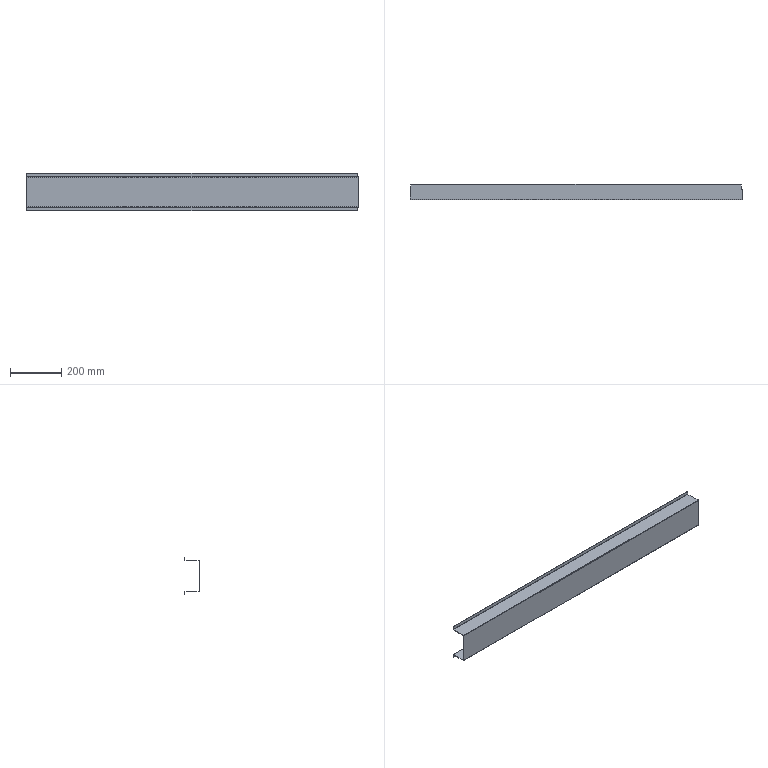Part | SolidWorks | features EdgeFlange 2, FlatPattern 1, ICE 1, SMBaseFlange 1, SheetMetal 1 | 1 solid | 38 faces | box 1298 x 58.8 x 147.6 mm | volume 406084 mm3 | plane 30 | cylinder 8 | commonest cylinder face diameters 0.9 x4 3.3 x4
STEP:
#1=CARTESIAN_POINT('',(646.8,57.15,60.));
#2=VERTEX_POINT('',#1);
#3=CARTESIAN_POINT('',(646.8,38.8,60.));
#4=VERTEX_POINT('',#3);
#5=CARTESIAN_POINT('',(646.8,58.8,60.));
#6=DIRECTION('',(0.,-1.,0.));
#7=VECTOR('',#6,1000.);
#8=LINE('',#5,#7);
#9=EDGE_CURVE('',#2,#4,#8,.T.);
#10=ORIENTED_EDGE('',*,*,#9,.F.);
#11=CARTESIAN_POINT('',(-646.8,57.15,60.));
#12=VERTEX_POINT('',#11);
#13=CARTESIAN_POINT('',(-648.8,57.15,60.));
#14=DIRECTION('',(1.,0.,0.));
#15=VECTOR('',#14,1000.);
#16=LINE('',#13,#15);
#17=EDGE_CURVE('',#12,#2,#16,.T.);
#18=ORIENTED_EDGE('',*,*,#17,.F.);
#19=CARTESIAN_POINT('',(-646.8,38.8,60.));
#20=VERTEX_POINT('',#19);
#21=CARTESIAN_POINT('',(-646.8,58.8,60.));
#22=DIRECTION('',(0.,1.,0.));
#23=VECTOR('',#22,1000.);
#24=LINE('',#21,#23);
#25=EDGE_CURVE('',#20,#12,#24,.T.);
#26=ORIENTED_EDGE('',*,*,#25,.F.);
#27=CARTESIAN_POINT('',(-648.8,38.8,60.));
#28=VERTEX_POINT('',#27);
#29=CARTESIAN_POINT('',(-648.8,38.8,60.));
#30=DIRECTION('',(1.,0.,0.));
#31=VECTOR('',#30,1000.);
#32=LINE('',#29,#31);
#33=EDGE_CURVE('',#28,#20,#32,.T.);
#34=ORIENTED_EDGE('',*,*,#33,.F.);
#35=CARTESIAN_POINT('',(-648.8,1.65,60.));
#36=VERTEX_POINT('',#35);
#37=CARTESIAN_POINT('',(-648.8,58.8,60.));
#38=DIRECTION('',(0.,-1.,0.));
#39=VECTOR('',#38,1000.);
#40=LINE('',#37,#39);
#41=EDGE_CURVE('',#28,#36,#40,.T.);
#42=ORIENTED_EDGE('',*,*,#41,.T.);
#43=CARTESIAN_POINT('',(648.8,1.65,60.));
#44=VERTEX_POINT('',#43);
#45=CARTESIAN_POINT('',(-648.8,1.65,60.));
#46=DIRECTION('',(-1.,0.,0.));
#47=VECTOR('',#46,1000.);
#48=LINE('',#45,#47);
#49=EDGE_CURVE('',#44,#36,#48,.T.);
#50=ORIENTED_EDGE('',*,*,#49,.F.);
#51=CARTESIAN_POINT('',(648.8,38.8,60.));
#52=VERTEX_POINT('',#51);
#53=CARTESIAN_POINT('',(648.8,58.8,60.));
#54=DIRECTION('',(0.,1.,0.));
#55=VECTOR('',#54,1000.);
#56=LINE('',#53,#55);
#57=EDGE_CURVE('',#44,#52,#56,.T.);
#58=ORIENTED_EDGE('',*,*,#57,.T.);
#59=CARTESIAN_POINT('',(-648.8,38.8,60.));
#60=DIRECTION('',(1.,0.,0.));
#61=VECTOR('',#60,1000.);
#62=LINE('',#59,#61);
#63=EDGE_CURVE('',#4,#52,#62,.T.);
#64=ORIENTED_EDGE('',*,*,#63,.F.);
#65=EDGE_LOOP('',(#10,#18,#26,#34,#42,#50,#58,#64));
#66=FACE_OUTER_BOUND('',#65,.T.);
#67=CARTESIAN_POINT('',(-648.8,58.8,60.));
#68=DIRECTION('',(0.,0.,-1.));
#69=DIRECTION('',(-1.,0.,0.));
#70=AXIS2_PLACEMENT_3D('',#67,#68,#69);
#71=PLANE('',#70);
#72=ADVANCED_FACE('',(#66),#71,.F.);
#73=CARTESIAN_POINT('',(-646.8,57.15,58.8));
#74=VERTEX_POINT('',#73);
#75=CARTESIAN_POINT('',(646.8,57.15,58.8));
#76=VERTEX_POINT('',#75);
#77=CARTESIAN_POINT('',(-648.8,57.15,58.8));
#78=DIRECTION('',(1.,0.,0.));
#79=VECTOR('',#78,1000.);
#80=LINE('',#77,#79);
#81=EDGE_CURVE('',#74,#76,#80,.T.);
#82=ORIENTED_EDGE('',*,*,#81,.T.);
#83=CARTESIAN_POINT('',(646.8,38.8,58.8));
#84=VERTEX_POINT('',#83);
#85=CARTESIAN_POINT('',(646.8,58.8,58.8));
#86=DIRECTION('',(0.,-1.,0.));
#87=VECTOR('',#86,1000.);
#88=LINE('',#85,#87);
#89=EDGE_CURVE('',#76,#84,#88,.T.);
#90=ORIENTED_EDGE('',*,*,#89,.T.);
#91=CARTESIAN_POINT('',(648.8,38.8,58.8));
#92=VERTEX_POINT('',#91);
#93=CARTESIAN_POINT('',(-648.8,38.8,58.8));
#94=DIRECTION('',(1.,0.,0.));
#95=VECTOR('',#94,1000.);
#96=LINE('',#93,#95);
#97=EDGE_CURVE('',#84,#92,#96,.T.);
#98=ORIENTED_EDGE('',*,*,#97,.T.);
#99=CARTESIAN_POINT('',(648.8,1.65,58.8));
#100=VERTEX_POINT('',#99);
#101=CARTESIAN_POINT('',(648.8,58.8,58.8));
#102=DIRECTION('',(0.,1.,0.));
#103=VECTOR('',#102,1000.);
#104=LINE('',#101,#103);
#105=EDGE_CURVE('',#100,#92,#104,.T.);
#106=ORIENTED_EDGE('',*,*,#105,.F.);
#107=CARTESIAN_POINT('',(-648.8,1.65,58.8));
#108=VERTEX_POINT('',#107);
#109=CARTESIAN_POINT('',(-648.8,1.65,58.8));
#110=DIRECTION('',(1.,0.,0.));
#111=VECTOR('',#110,1000.);
#112=LINE('',#109,#111);
#113=EDGE_CURVE('',#108,#100,#112,.T.);
#114=ORIENTED_EDGE('',*,*,#113,.F.);
#115=CARTESIAN_POINT('',(-648.8,38.8,58.8));
#116=VERTEX_POINT('',#115);
#117=CARTESIAN_POINT('',(-648.8,1.2,58.8));
#118=DIRECTION('',(0.,-1.,0.));
#119=VECTOR('',#118,1000.);
#120=LINE('',#117,#119);
#121=EDGE_CURVE('',#116,#108,#120,.T.);
#122=ORIENTED_EDGE('',*,*,#121,.F.);
#123=CARTESIAN_POINT('',(-646.8,38.8,58.8));
#124=VERTEX_POINT('',#123);
#125=CARTESIAN_POINT('',(-648.8,38.8,58.8));
#126=DIRECTION('',(1.,0.,0.));
#127=VECTOR('',#126,1000.);
#128=LINE('',#125,#127);
#129=EDGE_CURVE('',#116,#124,#128,.T.);
#130=ORIENTED_EDGE('',*,*,#129,.T.);
#131=CARTESIAN_POINT('',(-646.8,58.8,58.8));
#132=DIRECTION('',(0.,1.,0.));
#133=VECTOR('',#132,1000.);
#134=LINE('',#131,#133);
#135=EDGE_CURVE('',#124,#74,#134,.T.);
#136=ORIENTED_EDGE('',*,*,#135,.T.);
#137=EDGE_LOOP('',(#82,#90,#98,#106,#114,#122,#130,#136));
#138=FACE_OUTER_BOUND('',#137,.T.);
#139=CARTESIAN_POINT('',(-648.8,58.8,58.8));
#140=DIRECTION('',(0.,0.,-1.));
#141=DIRECTION('',(-1.,0.,0.));
#142=AXIS2_PLACEMENT_3D('',#139,#140,#141);
#143=PLANE('',#142);
#144=ADVANCED_FACE('',(#138),#143,.T.);
#145=CARTESIAN_POINT('',(646.8,38.8,-60.));
#146=VERTEX_POINT('',#145);
#147=CARTESIAN_POINT('',(646.8,57.15,-60.));
#148=VERTEX_POINT('',#147);
#149=CARTESIAN_POINT('',(646.8,58.8,-60.));
#150=DIRECTION('',(0.,1.,0.));
#151=VECTOR('',#150,1000.);
#152=LINE('',#149,#151);
#153=EDGE_CURVE('',#146,#148,#152,.T.);
#154=ORIENTED_EDGE('',*,*,#153,.F.);
#155=CARTESIAN_POINT('',(648.8,38.8,-60.));
#156=VERTEX_POINT('',#155);
#157=CARTESIAN_POINT('',(648.8,38.8,-60.));
#158=DIRECTION('',(-1.,0.,0.));
#159=VECTOR('',#158,1000.);
#160=LINE('',#157,#159);
#161=EDGE_CURVE('',#156,#146,#160,.T.);
#162=ORIENTED_EDGE('',*,*,#161,.F.);
#163=CARTESIAN_POINT('',(648.8,1.65,-60.));
#164=VERTEX_POINT('',#163);
#165=CARTESIAN_POINT('',(648.8,58.8,-60.));
#166=DIRECTION('',(0.,-1.,0.));
#167=VECTOR('',#166,1000.);
#168=LINE('',#165,#167);
#169=EDGE_CURVE('',#156,#164,#168,.T.);
#170=ORIENTED_EDGE('',*,*,#169,.T.);
#171=CARTESIAN_POINT('',(-648.8,1.65,-60.));
#172=VERTEX_POINT('',#171);
#173=CARTESIAN_POINT('',(648.8,1.65,-60.));
#174=DIRECTION('',(1.,0.,0.));
#175=VECTOR('',#174,1000.);
#176=LINE('',#173,#175);
#177=EDGE_CURVE('',#172,#164,#176,.T.);
#178=ORIENTED_EDGE('',*,*,#177,.F.);
#179=CARTESIAN_POINT('',(-648.8,38.8,-60.));
#180=VERTEX_POINT('',#179);
#181=CARTESIAN_POINT('',(-648.8,58.8,-60.));
#182=DIRECTION('',(0.,1.,0.));
#183=VECTOR('',#182,1000.);
#184=LINE('',#181,#183);
#185=EDGE_CURVE('',#172,#180,#184,.T.);
#186=ORIENTED_EDGE('',*,*,#185,.T.);
#187=CARTESIAN_POINT('',(-646.8,38.8,-60.));
#188=VERTEX_POINT('',#187);
#189=CARTESIAN_POINT('',(648.8,38.8,-60.));
#190=DIRECTION('',(-1.,0.,0.));
#191=VECTOR('',#190,1000.);
#192=LINE('',#189,#191);
#193=EDGE_CURVE('',#188,#180,#192,.T.);
#194=ORIENTED_EDGE('',*,*,#193,.F.);
#195=CARTESIAN_POINT('',(-646.8,57.15,-60.));
#196=VERTEX_POINT('',#195);
#197=CARTESIAN_POINT('',(-646.8,58.8,-60.));
#198=DIRECTION('',(0.,-1.,0.));
#199=VECTOR('',#198,1000.);
#200=LINE('',#197,#199);
#201=EDGE_CURVE('',#196,#188,#200,.T.);
#202=ORIENTED_EDGE('',*,*,#201,.F.);
#203=CARTESIAN_POINT('',(648.8,57.15,-60.));
#204=DIRECTION('',(-1.,0.,0.));
#205=VECTOR('',#204,1000.);
#206=LINE('',#203,#205);
#207=EDGE_CURVE('',#148,#196,#206,.T.);
#208=ORIENTED_EDGE('',*,*,#207,.F.);
#209=EDGE_LOOP('',(#154,#162,#170,#178,#186,#194,#202,#208));
#210=FACE_OUTER_BOUND('',#209,.T.);
#211=CARTESIAN_POINT('',(648.8,58.8,-60.));
#212=DIRECTION('',(0.,0.,1.));
#213=DIRECTION('',(0.,-1.,0.));
#214=AXIS2_PLACEMENT_3D('',#211,#212,#213);
#215=PLANE('',#214);
#216=ADVANCED_FACE('',(#210),#215,.F.);
#217=CARTESIAN_POINT('',(648.8,38.8,-58.8));
#218=VERTEX_POINT('',#217);
#219=CARTESIAN_POINT('',(646.8,38.8,-58.8));
#220=VERTEX_POINT('',#219);
#221=CARTESIAN_POINT('',(648.8,38.8,-58.8));
#222=DIRECTION('',(-1.,0.,0.));
#223=VECTOR('',#222,1000.);
#224=LINE('',#221,#223);
#225=EDGE_CURVE('',#218,#220,#224,.T.);
#226=ORIENTED_EDGE('',*,*,#225,.T.);
#227=CARTESIAN_POINT('',(646.8,57.15,-58.8));
#228=VERTEX_POINT('',#227);
#229=CARTESIAN_POINT('',(646.8,58.8,-58.8));
#230=DIRECTION('',(0.,1.,0.));
#231=VECTOR('',#230,1000.);
#232=LINE('',#229,#231);
#233=EDGE_CURVE('',#220,#228,#232,.T.);
#234=ORIENTED_EDGE('',*,*,#233,.T.);
#235=CARTESIAN_POINT('',(-646.8,57.15,-58.8));
#236=VERTEX_POINT('',#235);
#237=CARTESIAN_POINT('',(648.8,57.15,-58.8));
#238=DIRECTION('',(-1.,0.,0.));
#239=VECTOR('',#238,1000.);
#240=LINE('',#237,#239);
#241=EDGE_CURVE('',#228,#236,#240,.T.);
#242=ORIENTED_EDGE('',*,*,#241,.T.);
#243=CARTESIAN_POINT('',(-646.8,38.8,-58.8));
#244=VERTEX_POINT('',#243);
#245=CARTESIAN_POINT('',(-646.8,58.8,-58.8));
#246=DIRECTION('',(0.,-1.,0.));
#247=VECTOR('',#246,1000.);
#248=LINE('',#245,#247);
#249=EDGE_CURVE('',#236,#244,#248,.T.);
#250=ORIENTED_EDGE('',*,*,#249,.T.);
#251=CARTESIAN_POINT('',(-648.8,38.8,-58.8));
#252=VERTEX_POINT('',#251);
#253=CARTESIAN_POINT('',(648.8,38.8,-58.8));
#254=DIRECTION('',(-1.,0.,0.));
#255=VECTOR('',#254,1000.);
#256=LINE('',#253,#255);
#257=EDGE_CURVE('',#244,#252,#256,.T.);
#258=ORIENTED_EDGE('',*,*,#257,.T.);
#259=CARTESIAN_POINT('',(-648.8,1.65,-58.8));
#260=VERTEX_POINT('',#259);
#261=CARTESIAN_POINT('',(-648.8,58.8,-58.8));
#262=DIRECTION('',(0.,1.,0.));
#263=VECTOR('',#262,1000.);
#264=LINE('',#261,#263);
#265=EDGE_CURVE('',#260,#252,#264,.T.);
#266=ORIENTED_EDGE('',*,*,#265,.F.);
#267=CARTESIAN_POINT('',(648.8,1.65,-58.8));
#268=VERTEX_POINT('',#267);
#269=CARTESIAN_POINT('',(648.8,1.65,-58.8));
#270=DIRECTION('',(-1.,0.,0.));
#271=VECTOR('',#270,1000.);
#272=LINE('',#269,#271);
#273=EDGE_CURVE('',#268,#260,#272,.T.);
#274=ORIENTED_EDGE('',*,*,#273,.F.);
#275=CARTESIAN_POINT('',(648.8,1.2,-58.8));
#276=DIRECTION('',(0.,-1.,0.));
#277=VECTOR('',#276,1000.);
#278=LINE('',#275,#277);
#279=EDGE_CURVE('',#218,#268,#278,.T.);
#280=ORIENTED_EDGE('',*,*,#279,.F.);
#281=EDGE_LOOP('',(#226,#234,#242,#250,#258,#266,#274,#280));
#282=FACE_OUTER_BOUND('',#281,.T.);
#283=CARTESIAN_POINT('',(648.8,58.8,-58.8));
#284=DIRECTION('',(0.,0.,1.));
#285=DIRECTION('',(0.,-1.,0.));
#286=AXIS2_PLACEMENT_3D('',#283,#284,#285);
#287=PLANE('',#286);
#288=ADVANCED_FACE('',(#282),#287,.T.);
#289=ORIENTED_EDGE('',*,*,#241,.F.);
#290=CARTESIAN_POINT('',(646.8,58.8,-60.45));
#291=VERTEX_POINT('',#290);
#292=CARTESIAN_POINT('',(646.8,57.15,-60.45));
#293=DIRECTION('',(-1.,0.,0.));
#294=DIRECTION('',(0.,0.,-1.));
#295=AXIS2_PLACEMENT_3D('',#292,#293,#294);
#296=CIRCLE('',#295,1.65);
#297=EDGE_CURVE('',#228,#291,#296,.T.);
#298=ORIENTED_EDGE('',*,*,#297,.T.);
#299=CARTESIAN_POINT('',(-646.8,58.8,-60.45));
#300=VERTEX_POINT('',#299);
#301=CARTESIAN_POINT('',(648.8,58.8,-60.45));
#302=DIRECTION('',(1.,0.,0.));
#303=VECTOR('',#302,1000.);
#304=LINE('',#301,#303);
#305=EDGE_CURVE('',#300,#291,#304,.T.);
#306=ORIENTED_EDGE('',*,*,#305,.F.);
#307=CARTESIAN_POINT('',(-646.8,57.15,-60.45));
#308=DIRECTION('',(1.,0.,0.));
#309=DIRECTION('',(0.,0.,1.));
#310=AXIS2_PLACEMENT_3D('',#307,#308,#309);
#311=CIRCLE('',#310,1.65);
#312=EDGE_CURVE('',#300,#236,#311,.T.);
#313=ORIENTED_EDGE('',*,*,#312,.T.);
#314=EDGE_LOOP('',(#289,#298,#306,#313));
#315=FACE_OUTER_BOUND('',#314,.T.);
#316=CARTESIAN_POINT('',(648.8,57.15,-60.45));
#317=DIRECTION('',(1.,0.,0.));
#318=DIRECTION('',(0.,1.,0.));
#319=AXIS2_PLACEMENT_3D('',#316,#317,#318);
#320=CYLINDRICAL_SURFACE('',#319,1.65);
#321=ADVANCED_FACE('',(#315),#320,.T.);
#322=CARTESIAN_POINT('',(646.8,57.6,-60.45));
#323=VERTEX_POINT('',#322);
#324=CARTESIAN_POINT('',(646.8,57.15,-60.45));
#325=DIRECTION('',(-1.,0.,0.));
#326=DIRECTION('',(0.,0.,-1.));
#327=AXIS2_PLACEMENT_3D('',#324,#325,#326);
#328=CIRCLE('',#327,0.45);
#329=EDGE_CURVE('',#148,#323,#328,.T.);
#330=ORIENTED_EDGE('',*,*,#329,.F.);
#331=ORIENTED_EDGE('',*,*,#207,.T.);
#332=CARTESIAN_POINT('',(-646.8,57.6,-60.45));
#333=VERTEX_POINT('',#332);
#334=CARTESIAN_POINT('',(-646.8,57.15,-60.45));
#335=DIRECTION('',(1.,0.,0.));
#336=DIRECTION('',(0.,0.,1.));
#337=AXIS2_PLACEMENT_3D('',#334,#335,#336);
#338=CIRCLE('',#337,0.45);
#339=EDGE_CURVE('',#333,#196,#338,.T.);
#340=ORIENTED_EDGE('',*,*,#339,.F.);
#341=CARTESIAN_POINT('',(-648.8,57.6,-60.45));
#342=DIRECTION('',(1.,0.,0.));
#343=VECTOR('',#342,1000.);
#344=LINE('',#341,#343);
#345=EDGE_CURVE('',#333,#323,#344,.T.);
#346=ORIENTED_EDGE('',*,*,#345,.T.);
#347=EDGE_LOOP('',(#330,#331,#340,#346));
#348=FACE_OUTER_BOUND('',#347,.T.);
#349=CARTESIAN_POINT('',(648.8,57.15,-60.45));
#350=DIRECTION('',(1.,0.,0.));
#351=DIRECTION('',(0.,1.,0.));
#352=AXIS2_PLACEMENT_3D('',#349,#350,#351);
#353=CYLINDRICAL_SURFACE('',#352,0.45);
#354=ADVANCED_FACE('',(#348),#353,.F.);
#355=ORIENTED_EDGE('',*,*,#305,.T.);
#356=CARTESIAN_POINT('',(646.8,58.8,-73.8));
#357=VERTEX_POINT('',#356);
#358=CARTESIAN_POINT('',(646.8,58.8,140.));
#359=DIRECTION('',(0.,0.,-1.));
#360=VECTOR('',#359,1000.);
#361=LINE('',#358,#360);
#362=EDGE_CURVE('',#291,#357,#361,.T.);
#363=ORIENTED_EDGE('',*,*,#362,.T.);
#364=CARTESIAN_POINT('',(-646.8,58.8,-73.8));
#365=VERTEX_POINT('',#364);
#366=CARTESIAN_POINT('',(648.8,58.8,-73.8));
#367=DIRECTION('',(1.,0.,0.));
#368=VECTOR('',#367,1000.);
#369=LINE('',#366,#368);
#370=EDGE_CURVE('',#365,#357,#369,.T.);
#371=ORIENTED_EDGE('',*,*,#370,.F.);
#372=CARTESIAN_POINT('',(-646.8,58.8,140.));
#373=DIRECTION('',(0.,0.,-1.));
#374=VECTOR('',#373,1000.);
#375=LINE('',#372,#374);
#376=EDGE_CURVE('',#300,#365,#375,.T.);
#377=ORIENTED_EDGE('',*,*,#376,.F.);
#378=EDGE_LOOP('',(#355,#363,#371,#377));
#379=FACE_OUTER_BOUND('',#378,.T.);
#380=CARTESIAN_POINT('',(648.8,58.8,-60.));
#381=DIRECTION('',(0.,1.,0.));
#382=DIRECTION('',(0.,0.,1.));
#383=AXIS2_PLACEMENT_3D('',#380,#381,#382);
#384=PLANE('',#383);
#385=ADVANCED_FACE('',(#379),#384,.T.);
#386=CARTESIAN_POINT('',(646.8,57.6,-73.8));
#387=VERTEX_POINT('',#386);
#388=CARTESIAN_POINT('',(646.8,57.6,-60.));
#389=DIRECTION('',(0.,0.,-1.));
#390=VECTOR('',#389,1000.);
#391=LINE('',#388,#390);
#392=EDGE_CURVE('',#323,#387,#391,.T.);
#393=ORIENTED_EDGE('',*,*,#392,.F.);
#394=ORIENTED_EDGE('',*,*,#345,.F.);
#395=CARTESIAN_POINT('',(-646.8,57.6,-73.8));
#396=VERTEX_POINT('',#395);
#397=CARTESIAN_POINT('',(-646.8,57.6,-60.));
#398=DIRECTION('',(0.,0.,1.));
#399=VECTOR('',#398,1000.);
#400=LINE('',#397,#399);
#401=EDGE_CURVE('',#396,#333,#400,.T.);
#402=ORIENTED_EDGE('',*,*,#401,.F.);
#403=CARTESIAN_POINT('',(648.8,57.6,-73.8));
#404=DIRECTION('',(1.,0.,0.));
#405=VECTOR('',#404,1000.);
#406=LINE('',#403,#405);
#407=EDGE_CURVE('',#396,#387,#406,.T.);
#408=ORIENTED_EDGE('',*,*,#407,.T.);
#409=EDGE_LOOP('',(#393,#394,#402,#408));
#410=FACE_OUTER_BOUND('',#409,.T.);
#411=CARTESIAN_POINT('',(648.8,57.6,-60.));
#412=DIRECTION('',(0.,1.,0.));
#413=DIRECTION('',(0.,0.,1.));
#414=AXIS2_PLACEMENT_3D('',#411,#412,#413);
#415=PLANE('',#414);
#416=ADVANCED_FACE('',(#410),#415,.F.);
#417=ORIENTED_EDGE('',*,*,#370,.T.);
#418=CARTESIAN_POINT('',(646.8,58.8,-73.8));
#419=DIRECTION('',(0.,-1.,0.));
#420=VECTOR('',#419,1000.);
#421=LINE('',#418,#420);
#422=EDGE_CURVE('',#357,#387,#421,.T.);
#423=ORIENTED_EDGE('',*,*,#422,.T.);
#424=ORIENTED_EDGE('',*,*,#407,.F.);
#425=CARTESIAN_POINT('',(-646.8,58.8,-73.8));
#426=DIRECTION('',(0.,1.,0.));
#427=VECTOR('',#426,1000.);
#428=LINE('',#425,#427);
#429=EDGE_CURVE('',#396,#365,#428,.T.);
#430=ORIENTED_EDGE('',*,*,#429,.T.);
#431=EDGE_LOOP('',(#417,#423,#424,#430));
#432=FACE_OUTER_BOUND('',#431,.T.);
#433=CARTESIAN_POINT('',(648.8,58.8,-73.8));
#434=DIRECTION('',(0.,0.,-1.));
#435=DIRECTION('',(0.,1.,0.));
#436=AXIS2_PLACEMENT_3D('',#433,#434,#435);
#437=PLANE('',#436);
#438=ADVANCED_FACE('',(#432),#437,.T.);
#439=CARTESIAN_POINT('',(-646.8,58.8,60.45));
#440=VERTEX_POINT('',#439);
#441=CARTESIAN_POINT('',(646.8,58.8,60.45));
#442=VERTEX_POINT('',#441);
#443=CARTESIAN_POINT('',(648.8,58.8,60.45));
#444=DIRECTION('',(1.,0.,0.));
#445=VECTOR('',#444,1000.);
#446=LINE('',#443,#445);
#447=EDGE_CURVE('',#440,#442,#446,.T.);
#448=ORIENTED_EDGE('',*,*,#447,.T.);
#449=CARTESIAN_POINT('',(646.8,57.15,60.45));
#450=DIRECTION('',(-1.,0.,0.));
#451=DIRECTION('',(0.,0.,-1.));
#452=AXIS2_PLACEMENT_3D('',#449,#450,#451);
#453=CIRCLE('',#452,1.65);
#454=EDGE_CURVE('',#442,#76,#453,.T.);
#455=ORIENTED_EDGE('',*,*,#454,.T.);
#456=ORIENTED_EDGE('',*,*,#81,.F.);
#457=CARTESIAN_POINT('',(-646.8,57.15,60.45));
#458=DIRECTION('',(1.,0.,0.));
#459=DIRECTION('',(0.,0.,1.));
#460=AXIS2_PLACEMENT_3D('',#457,#458,#459);
#461=CIRCLE('',#460,1.65);
#462=EDGE_CURVE('',#74,#440,#461,.T.);
#463=ORIENTED_EDGE('',*,*,#462,.T.);
#464=EDGE_LOOP('',(#448,#455,#456,#463));
#465=FACE_OUTER_BOUND('',#464,.T.);
#466=CARTESIAN_POINT('',(-648.8,57.15,60.45));
#467=DIRECTION('',(-1.,0.,0.));
#468=DIRECTION('',(0.,1.,0.));
#469=AXIS2_PLACEMENT_3D('',#466,#467,#468);
#470=CYLINDRICAL_SURFACE('',#469,1.65);
#471=ADVANCED_FACE('',(#465),#470,.T.);
#472=CARTESIAN_POINT('',(646.8,57.6,60.45));
#473=VERTEX_POINT('',#472);
#474=CARTESIAN_POINT('',(646.8,57.15,60.45));
#475=DIRECTION('',(-1.,0.,0.));
#476=DIRECTION('',(0.,0.,-1.));
#477=AXIS2_PLACEMENT_3D('',#474,#475,#476);
#478=CIRCLE('',#477,0.45);
#479=EDGE_CURVE('',#473,#2,#478,.T.);
#480=ORIENTED_EDGE('',*,*,#479,.F.);
#481=CARTESIAN_POINT('',(-646.8,57.6,60.45));
#482=VERTEX_POINT('',#481);
#483=CARTESIAN_POINT('',(648.8,57.6,60.45));
#484=DIRECTION('',(-1.,0.,0.));
#485=VECTOR('',#484,1000.);
#486=LINE('',#483,#485);
#487=EDGE_CURVE('',#473,#482,#486,.T.);
#488=ORIENTED_EDGE('',*,*,#487,.T.);
#489=CARTESIAN_POINT('',(-646.8,57.15,60.45));
#490=DIRECTION('',(1.,0.,0.));
#491=DIRECTION('',(0.,0.,1.));
#492=AXIS2_PLACEMENT_3D('',#489,#490,#491);
#493=CIRCLE('',#492,0.45);
#494=EDGE_CURVE('',#12,#482,#493,.T.);
#495=ORIENTED_EDGE('',*,*,#494,.F.);
#496=ORIENTED_EDGE('',*,*,#17,.T.);
#497=EDGE_LOOP('',(#480,#488,#495,#496));
#498=FACE_OUTER_BOUND('',#497,.T.);
#499=CARTESIAN_POINT('',(-648.8,57.15,60.45));
#500=DIRECTION('',(-1.,0.,0.));
#501=DIRECTION('',(0.,1.,0.));
#502=AXIS2_PLACEMENT_3D('',#499,#500,#501);
#503=CYLINDRICAL_SURFACE('',#502,0.45);
#504=ADVANCED_FACE('',(#498),#503,.F.);
#505=CARTESIAN_POINT('',(646.8,58.8,73.8));
#506=VERTEX_POINT('',#505);
#507=CARTESIAN_POINT('',(646.8,58.8,140.));
#508=DIRECTION('',(0.,0.,-1.));
#509=VECTOR('',#508,1000.);
#510=LINE('',#507,#509);
#511=EDGE_CURVE('',#506,#442,#510,.T.);
#512=ORIENTED_EDGE('',*,*,#511,.T.);
#513=ORIENTED_EDGE('',*,*,#447,.F.);
#514=CARTESIAN_POINT('',(-646.8,58.8,73.8));
#515=VERTEX_POINT('',#514);
#516=CARTESIAN_POINT('',(-646.8,58.8,140.));
#517=DIRECTION('',(0.,0.,-1.));
#518=VECTOR('',#517,1000.);
#519=LINE('',#516,#518);
#520=EDGE_CURVE('',#515,#440,#519,.T.);
#521=ORIENTED_EDGE('',*,*,#520,.F.);
#522=CARTESIAN_POINT('',(648.8,58.8,73.8));
#523=DIRECTION('',(-1.,0.,0.));
#524=VECTOR('',#523,1000.);
#525=LINE('',#522,#524);
#526=EDGE_CURVE('',#506,#515,#525,.T.);
#527=ORIENTED_EDGE('',*,*,#526,.F.);
#528=EDGE_LOOP('',(#512,#513,#521,#527));
#529=FACE_OUTER_BOUND('',#528,.T.);
#530=CARTESIAN_POINT('',(648.8,58.8,73.8));
#531=DIRECTION('',(0.,-1.,0.));
#532=DIRECTION('',(0.,0.,-1.));
#533=AXIS2_PLACEMENT_3D('',#530,#531,#532);
#534=PLANE('',#533);
#535=ADVANCED_FACE('',(#529),#534,.F.);
#536=ORIENTED_EDGE('',*,*,#487,.F.);
#537=CARTESIAN_POINT('',(646.8,57.6,73.8));
#538=VERTEX_POINT('',#537);
#539=CARTESIAN_POINT('',(646.8,57.6,73.8));
#540=DIRECTION('',(0.,0.,1.));
#541=VECTOR('',#540,1000.);
#542=LINE('',#539,#541);
#543=EDGE_CURVE('',#473,#538,#542,.T.);
#544=ORIENTED_EDGE('',*,*,#543,.T.);
#545=CARTESIAN_POINT('',(-646.8,57.6,73.8));
#546=VERTEX_POINT('',#545);
#547=CARTESIAN_POINT('',(648.8,57.6,73.8));
#548=DIRECTION('',(-1.,0.,0.));
#549=VECTOR('',#548,1000.);
#550=LINE('',#547,#549);
#551=EDGE_CURVE('',#538,#546,#550,.T.);
#552=ORIENTED_EDGE('',*,*,#551,.T.);
#553=CARTESIAN_POINT('',(-646.8,57.6,73.8));
#554=DIRECTION('',(0.,0.,-1.));
#555=VECTOR('',#554,1000.);
#556=LINE('',#553,#555);
#557=EDGE_CURVE('',#546,#482,#556,.T.);
#558=ORIENTED_EDGE('',*,*,#557,.T.);
#559=EDGE_LOOP('',(#536,#544,#552,#558));
#560=FACE_OUTER_BOUND('',#559,.T.);
#561=CARTESIAN_POINT('',(648.8,57.6,73.8));
#562=DIRECTION('',(0.,-1.,0.));
#563=DIRECTION('',(0.,0.,-1.));
#564=AXIS2_PLACEMENT_3D('',#561,#562,#563);
#565=PLANE('',#564);
#566=ADVANCED_FACE('',(#560),#565,.T.);
#567=ORIENTED_EDGE('',*,*,#551,.F.);
#568=CARTESIAN_POINT('',(646.8,58.8,73.8));
#569=DIRECTION('',(0.,1.,0.));
#570=VECTOR('',#569,1000.);
#571=LINE('',#568,#570);
#572=EDGE_CURVE('',#538,#506,#571,.T.);
#573=ORIENTED_EDGE('',*,*,#572,.T.);
#574=ORIENTED_EDGE('',*,*,#526,.T.);
#575=CARTESIAN_POINT('',(-646.8,58.8,73.8));
#576=DIRECTION('',(0.,-1.,0.));
#577=VECTOR('',#576,1000.);
#578=LINE('',#575,#577);
#579=EDGE_CURVE('',#515,#546,#578,.T.);
#580=ORIENTED_EDGE('',*,*,#579,.T.);
#581=EDGE_LOOP('',(#567,#573,#574,#580));
#582=FACE_OUTER_BOUND('',#581,.T.);
#583=CARTESIAN_POINT('',(648.8,58.8,73.8));
#584=DIRECTION('',(0.,0.,1.));
#585=DIRECTION('',(0.,-1.,0.));
#586=AXIS2_PLACEMENT_3D('',#583,#584,#585);
#587=PLANE('',#586);
#588=ADVANCED_FACE('',(#582),#587,.T.);
#589=CARTESIAN_POINT('',(648.8,38.8,140.));
#590=DIRECTION('',(0.,0.,-1.));
#591=VECTOR('',#590,1000.);
#592=LINE('',#589,#591);
#593=EDGE_CURVE('',#52,#92,#592,.T.);
#594=ORIENTED_EDGE('',*,*,#593,.F.);
#595=ORIENTED_EDGE('',*,*,#57,.F.);
#596=CARTESIAN_POINT('',(648.8,1.65,58.8));
#597=DIRECTION('',(0.,0.,1.));
#598=VECTOR('',#597,1000.);
#599=LINE('',#596,#598);
#600=EDGE_CURVE('',#100,#44,#599,.T.);
#601=ORIENTED_EDGE('',*,*,#600,.F.);
#602=ORIENTED_EDGE('',*,*,#105,.T.);
#603=EDGE_LOOP('',(#594,#595,#601,#602));
#604=FACE_OUTER_BOUND('',#603,.T.);
#605=CARTESIAN_POINT('',(648.8,58.8,60.));
#606=DIRECTION('',(-1.,0.,0.));
#607=DIRECTION('',(0.,0.,1.));
#608=AXIS2_PLACEMENT_3D('',#605,#606,#607);
#609=PLANE('',#608);
#610=ADVANCED_FACE('',(#604),#609,.F.);
#611=CARTESIAN_POINT('',(648.8,38.8,-60.));
#612=DIRECTION('',(0.,0.,-1.));
#613=VECTOR('',#612,1000.);
#614=LINE('',#611,#613);
#615=EDGE_CURVE('',#218,#156,#614,.T.);
#616=ORIENTED_EDGE('',*,*,#615,.F.);
#617=ORIENTED_EDGE('',*,*,#279,.T.);
#618=CARTESIAN_POINT('',(648.8,1.65,-60.));
#619=DIRECTION('',(0.,0.,-1.));
#620=VECTOR('',#619,1000.);
#621=LINE('',#618,#620);
#622=EDGE_CURVE('',#268,#164,#621,.T.);
#623=ORIENTED_EDGE('',*,*,#622,.T.);
#624=ORIENTED_EDGE('',*,*,#169,.F.);
#625=EDGE_LOOP('',(#616,#617,#623,#624));
#626=FACE_OUTER_BOUND('',#625,.T.);
#627=CARTESIAN_POINT('',(648.8,1.2,-60.));
#628=DIRECTION('',(-1.,0.,0.));
#629=DIRECTION('',(0.,0.,1.));
#630=AXIS2_PLACEMENT_3D('',#627,#628,#629);
#631=PLANE('',#630);
#632=ADVANCED_FACE('',(#626),#631,.F.);
#633=CARTESIAN_POINT('',(-648.8,38.8,140.));
#634=DIRECTION('',(0.,0.,-1.));
#635=VECTOR('',#634,1000.);
#636=LINE('',#633,#635);
#637=EDGE_CURVE('',#28,#116,#636,.T.);
#638=ORIENTED_EDGE('',*,*,#637,.T.);
#639=ORIENTED_EDGE('',*,*,#121,.T.);
#640=CARTESIAN_POINT('',(-648.8,1.65,60.));
#641=DIRECTION('',(0.,0.,1.));
#642=VECTOR('',#641,1000.);
#643=LINE('',#640,#642);
#644=EDGE_CURVE('',#108,#36,#643,.T.);
#645=ORIENTED_EDGE('',*,*,#644,.T.);
#646=ORIENTED_EDGE('',*,*,#41,.F.);
#647=EDGE_LOOP('',(#638,#639,#645,#646));
#648=FACE_OUTER_BOUND('',#647,.T.);
#649=CARTESIAN_POINT('',(-648.8,1.2,60.));
#650=DIRECTION('',(1.,0.,0.));
#651=DIRECTION('',(0.,0.,-1.));
#652=AXIS2_PLACEMENT_3D('',#649,#650,#651);
#653=PLANE('',#652);
#654=ADVANCED_FACE('',(#648),#653,.F.);
#655=CARTESIAN_POINT('',(-648.8,38.8,140.));
#656=DIRECTION('',(0.,0.,-1.));
#657=VECTOR('',#656,1000.);
#658=LINE('',#655,#657);
#659=EDGE_CURVE('',#252,#180,#658,.T.);
#660=ORIENTED_EDGE('',*,*,#659,.T.);
#661=ORIENTED_EDGE('',*,*,#185,.F.);
#662=CARTESIAN_POINT('',(-648.8,1.65,-58.8));
#663=DIRECTION('',(0.,0.,-1.));
#664=VECTOR('',#663,1000.);
#665=LINE('',#662,#664);
#666=EDGE_CURVE('',#260,#172,#665,.T.);
#667=ORIENTED_EDGE('',*,*,#666,.F.);
#668=ORIENTED_EDGE('',*,*,#265,.T.);
#669=EDGE_LOOP('',(#660,#661,#667,#668));
#670=FACE_OUTER_BOUND('',#669,.T.);
#671=CARTESIAN_POINT('',(-648.8,58.8,-60.));
#672=DIRECTION('',(1.,0.,0.));
#673=DIRECTION('',(0.,0.,-1.));
#674=AXIS2_PLACEMENT_3D('',#671,#672,#673);
#675=PLANE('',#674);
#676=ADVANCED_FACE('',(#670),#675,.F.);
#677=CARTESIAN_POINT('',(-648.8,1.2,58.35));
#678=VERTEX_POINT('',#677);
#679=CARTESIAN_POINT('',(-648.8,0.,58.35));
#680=VERTEX_POINT('',#679);
#681=CARTESIAN_POINT('',(-648.8,1.2,58.35));
#682=DIRECTION('',(0.,-1.,0.));
#683=VECTOR('',#682,1000.);
#684=LINE('',#681,#683);
#685=EDGE_CURVE('',#678,#680,#684,.T.);
#686=ORIENTED_EDGE('',*,*,#685,.F.);
#687=CARTESIAN_POINT('',(-648.8,1.2,-58.35));
#688=VERTEX_POINT('',#687);
#689=CARTESIAN_POINT('',(-648.8,1.2,-60.));
#690=DIRECTION('',(0.,0.,1.));
#691=VECTOR('',#690,1000.);
#692=LINE('',#689,#691);
#693=EDGE_CURVE('',#688,#678,#692,.T.);
#694=ORIENTED_EDGE('',*,*,#693,.F.);
#695=CARTESIAN_POINT('',(-648.8,0.,-58.35));
#696=VERTEX_POINT('',#695);
#697=CARTESIAN_POINT('',(-648.8,1.2,-58.35));
#698=DIRECTION('',(0.,-1.,0.));
#699=VECTOR('',#698,1000.);
#700=LINE('',#697,#699);
#701=EDGE_CURVE('',#688,#696,#700,.T.);
#702=ORIENTED_EDGE('',*,*,#701,.T.);
#703=CARTESIAN_POINT('',(-648.8,0.,-60.));
#704=DIRECTION('',(0.,0.,1.));
#705=VECTOR('',#704,1000.);
#706=LINE('',#703,#705);
#707=EDGE_CURVE('',#696,#680,#706,.T.);
#708=ORIENTED_EDGE('',*,*,#707,.T.);
#709=EDGE_LOOP('',(#686,#694,#702,#708));
#710=FACE_OUTER_BOUND('',#709,.T.);
#711=CARTESIAN_POINT('',(-648.8,1.2,-60.));
#712=DIRECTION('',(1.,0.,0.));
#713=DIRECTION('',(0.,0.,-1.));
#714=AXIS2_PLACEMENT_3D('',#711,#712,#713);
#715=PLANE('',#714);
#716=ADVANCED_FACE('',(#710),#715,.F.);
#717=CARTESIAN_POINT('',(648.8,1.2,58.35));
#718=VERTEX_POINT('',#717);
#719=CARTESIAN_POINT('',(648.8,0.,58.35));
#720=VERTEX_POINT('',#719);
#721=CARTESIAN_POINT('',(648.8,1.2,58.35));
#722=DIRECTION('',(0.,-1.,0.));
#723=VECTOR('',#722,1000.);
#724=LINE('',#721,#723);
#725=EDGE_CURVE('',#718,#720,#724,.T.);
#726=ORIENTED_EDGE('',*,*,#725,.T.);
#727=CARTESIAN_POINT('',(648.8,0.,-58.35));
#728=VERTEX_POINT('',#727);
#729=CARTESIAN_POINT('',(648.8,0.,-60.));
#730=DIRECTION('',(0.,0.,-1.));
#731=VECTOR('',#730,1000.);
#732=LINE('',#729,#731);
#733=EDGE_CURVE('',#720,#728,#732,.T.);
#734=ORIENTED_EDGE('',*,*,#733,.T.);
#735=CARTESIAN_POINT('',(648.8,1.2,-58.35));
#736=VERTEX_POINT('',#735);
#737=CARTESIAN_POINT('',(648.8,1.2,-58.35));
#738=DIRECTION('',(0.,-1.,0.));
#739=VECTOR('',#738,1000.);
#740=LINE('',#737,#739);
#741=EDGE_CURVE('',#736,#728,#740,.T.);
#742=ORIENTED_EDGE('',*,*,#741,.F.);
#743=CARTESIAN_POINT('',(648.8,1.2,-60.));
#744=DIRECTION('',(0.,0.,-1.));
#745=VECTOR('',#744,1000.);
#746=LINE('',#743,#745);
#747=EDGE_CURVE('',#718,#736,#746,.T.);
#748=ORIENTED_EDGE('',*,*,#747,.F.);
#749=EDGE_LOOP('',(#726,#734,#742,#748));
#750=FACE_OUTER_BOUND('',#749,.T.);
#751=CARTESIAN_POINT('',(648.8,1.2,-60.));
#752=DIRECTION('',(-1.,0.,0.));
#753=DIRECTION('',(0.,0.,1.));
#754=AXIS2_PLACEMENT_3D('',#751,#752,#753);
#755=PLANE('',#754);
#756=ADVANCED_FACE('',(#750),#755,.F.);
#757=ORIENTED_EDGE('',*,*,#693,.T.);
#758=CARTESIAN_POINT('',(648.8,1.2,58.35));
#759=DIRECTION('',(-1.,0.,0.));
#760=VECTOR('',#759,1000.);
#761=LINE('',#758,#760);
#762=EDGE_CURVE('',#718,#678,#761,.T.);
#763=ORIENTED_EDGE('',*,*,#762,.F.);
#764=ORIENTED_EDGE('',*,*,#747,.T.);
#765=CARTESIAN_POINT('',(-648.8,1.2,-58.35));
#766=DIRECTION('',(1.,0.,0.));
#767=VECTOR('',#766,1000.);
#768=LINE('',#765,#767);
#769=EDGE_CURVE('',#688,#736,#768,.T.);
#770=ORIENTED_EDGE('',*,*,#769,.F.);
#771=EDGE_LOOP('',(#757,#763,#764,#770));
#772=FACE_OUTER_BOUND('',#771,.T.);
#773=CARTESIAN_POINT('',(-648.8,1.2,60.));
#774=DIRECTION('',(0.,1.,0.));
#775=DIRECTION('',(0.,0.,1.));
#776=AXIS2_PLACEMENT_3D('',#773,#774,#775);
#777=PLANE('',#776);
#778=ADVANCED_FACE('',(#772),#777,.T.);
#779=CARTESIAN_POINT('',(648.8,0.,58.35));
#780=DIRECTION('',(-1.,0.,0.));
#781=VECTOR('',#780,1000.);
#782=LINE('',#779,#781);
#783=EDGE_CURVE('',#720,#680,#782,.T.);
#784=ORIENTED_EDGE('',*,*,#783,.T.);
#785=ORIENTED_EDGE('',*,*,#707,.F.);
#786=CARTESIAN_POINT('',(-648.8,0.,-58.35));
#787=DIRECTION('',(1.,0.,0.));
#788=VECTOR('',#787,1000.);
#789=LINE('',#786,#788);
#790=EDGE_CURVE('',#696,#728,#789,.T.);
#791=ORIENTED_EDGE('',*,*,#790,.T.);
#792=ORIENTED_EDGE('',*,*,#733,.F.);
#793=EDGE_LOOP('',(#784,#785,#791,#792));
#794=FACE_OUTER_BOUND('',#793,.T.);
#795=CARTESIAN_POINT('',(-648.8,0.,60.));
#796=DIRECTION('',(0.,1.,0.));
#797=DIRECTION('',(0.,0.,1.));
#798=AXIS2_PLACEMENT_3D('',#795,#796,#797);
#799=PLANE('',#798);
#800=ADVANCED_FACE('',(#794),#799,.F.);
#801=ORIENTED_EDGE('',*,*,#622,.F.);
#802=CARTESIAN_POINT('',(648.8,1.65,-58.35));
#803=DIRECTION('',(1.,0.,0.));
#804=DIRECTION('',(0.,-1.,0.));
#805=AXIS2_PLACEMENT_3D('',#802,#803,#804);
#806=CIRCLE('',#805,0.45);
#807=EDGE_CURVE('',#736,#268,#806,.T.);
#808=ORIENTED_EDGE('',*,*,#807,.F.);
#809=ORIENTED_EDGE('',*,*,#741,.T.);
#810=CARTESIAN_POINT('',(648.8,1.65,-58.35));
#811=DIRECTION('',(1.,0.,0.));
#812=DIRECTION('',(0.,-1.,0.));
#813=AXIS2_PLACEMENT_3D('',#810,#811,#812);
#814=CIRCLE('',#813,1.65);
#815=EDGE_CURVE('',#728,#164,#814,.T.);
#816=ORIENTED_EDGE('',*,*,#815,.T.);
#817=EDGE_LOOP('',(#801,#808,#809,#816));
#818=FACE_OUTER_BOUND('',#817,.T.);
#819=CARTESIAN_POINT('',(648.8,1.65,-58.35));
#820=DIRECTION('',(1.,0.,0.));
#821=DIRECTION('',(0.,1.,0.));
#822=AXIS2_PLACEMENT_3D('',#819,#820,#821);
#823=PLANE('',#822);
#824=ADVANCED_FACE('',(#818),#823,.T.);
#825=ORIENTED_EDGE('',*,*,#790,.F.);
#826=CARTESIAN_POINT('',(-648.8,1.65,-58.35));
#827=DIRECTION('',(-1.,0.,0.));
#828=DIRECTION('',(0.,-1.,0.));
#829=AXIS2_PLACEMENT_3D('',#826,#827,#828);
#830=CIRCLE('',#829,1.65);
#831=EDGE_CURVE('',#172,#696,#830,.T.);
#832=ORIENTED_EDGE('',*,*,#831,.F.);
#833=ORIENTED_EDGE('',*,*,#177,.T.);
#834=ORIENTED_EDGE('',*,*,#815,.F.);
#835=EDGE_LOOP('',(#825,#832,#833,#834));
#836=FACE_OUTER_BOUND('',#835,.T.);
#837=CARTESIAN_POINT('',(-648.8,1.65,-58.35));
#838=DIRECTION('',(-1.,0.,0.));
#839=DIRECTION('',(0.,0.,-1.));
#840=AXIS2_PLACEMENT_3D('',#837,#838,#839);
#841=CYLINDRICAL_SURFACE('',#840,1.65);
#842=ADVANCED_FACE('',(#836),#841,.T.);
#843=CARTESIAN_POINT('',(-648.8,1.65,-58.35));
#844=DIRECTION('',(-1.,0.,0.));
#845=DIRECTION('',(0.,-1.,0.));
#846=AXIS2_PLACEMENT_3D('',#843,#844,#845);
#847=CIRCLE('',#846,0.45);
#848=EDGE_CURVE('',#260,#688,#847,.T.);
#849=ORIENTED_EDGE('',*,*,#848,.F.);
#850=ORIENTED_EDGE('',*,*,#666,.T.);
#851=ORIENTED_EDGE('',*,*,#831,.T.);
#852=ORIENTED_EDGE('',*,*,#701,.F.);
#853=EDGE_LOOP('',(#849,#850,#851,#852));
#854=FACE_OUTER_BOUND('',#853,.T.);
#855=CARTESIAN_POINT('',(-648.8,1.65,-58.35));
#856=DIRECTION('',(1.,0.,0.));
#857=DIRECTION('',(0.,1.,0.));
#858=AXIS2_PLACEMENT_3D('',#855,#856,#857);
#859=PLANE('',#858);
#860=ADVANCED_FACE('',(#854),#859,.F.);
#861=ORIENTED_EDGE('',*,*,#769,.T.);
#862=ORIENTED_EDGE('',*,*,#807,.T.);
#863=ORIENTED_EDGE('',*,*,#273,.T.);
#864=ORIENTED_EDGE('',*,*,#848,.T.);
#865=EDGE_LOOP('',(#861,#862,#863,#864));
#866=FACE_OUTER_BOUND('',#865,.T.);
#867=CARTESIAN_POINT('',(-648.8,1.65,-58.35));
#868=DIRECTION('',(-1.,0.,0.));
#869=DIRECTION('',(0.,0.,-1.));
#870=AXIS2_PLACEMENT_3D('',#867,#868,#869);
#871=CYLINDRICAL_SURFACE('',#870,0.45);
#872=ADVANCED_FACE('',(#866),#871,.F.);
#873=ORIENTED_EDGE('',*,*,#644,.F.);
#874=CARTESIAN_POINT('',(-648.8,1.65,58.35));
#875=DIRECTION('',(-1.,0.,0.));
#876=DIRECTION('',(0.,0.,-1.));
#877=AXIS2_PLACEMENT_3D('',#874,#875,#876);
#878=CIRCLE('',#877,0.45);
#879=EDGE_CURVE('',#678,#108,#878,.T.);
#880=ORIENTED_EDGE('',*,*,#879,.F.);
#881=ORIENTED_EDGE('',*,*,#685,.T.);
#882=CARTESIAN_POINT('',(-648.8,1.65,58.35));
#883=DIRECTION('',(-1.,0.,0.));
#884=DIRECTION('',(0.,0.,-1.));
#885=AXIS2_PLACEMENT_3D('',#882,#883,#884);
#886=CIRCLE('',#885,1.65);
#887=EDGE_CURVE('',#680,#36,#886,.T.);
#888=ORIENTED_EDGE('',*,*,#887,.T.);
#889=EDGE_LOOP('',(#873,#880,#881,#888));
#890=FACE_OUTER_BOUND('',#889,.T.);
#891=CARTESIAN_POINT('',(-648.8,1.65,58.35));
#892=DIRECTION('',(-1.,0.,0.));
#893=DIRECTION('',(0.,0.,1.));
#894=AXIS2_PLACEMENT_3D('',#891,#892,#893);
#895=PLANE('',#894);
#896=ADVANCED_FACE('',(#890),#895,.T.);
#897=ORIENTED_EDGE('',*,*,#783,.F.);
#898=CARTESIAN_POINT('',(648.8,1.65,58.35));
#899=DIRECTION('',(1.,0.,0.));
#900=DIRECTION('',(0.,0.,-1.));
#901=AXIS2_PLACEMENT_3D('',#898,#899,#900);
#902=CIRCLE('',#901,1.65);
#903=EDGE_CURVE('',#44,#720,#902,.T.);
#904=ORIENTED_EDGE('',*,*,#903,.F.);
#905=ORIENTED_EDGE('',*,*,#49,.T.);
#906=ORIENTED_EDGE('',*,*,#887,.F.);
#907=EDGE_LOOP('',(#897,#904,#905,#906));
#908=FACE_OUTER_BOUND('',#907,.T.);
#909=CARTESIAN_POINT('',(648.8,1.65,58.35));
#910=DIRECTION('',(1.,0.,0.));
#911=DIRECTION('',(0.,0.,1.));
#912=AXIS2_PLACEMENT_3D('',#909,#910,#911);
#913=CYLINDRICAL_SURFACE('',#912,1.65);
#914=ADVANCED_FACE('',(#908),#913,.T.);
#915=CARTESIAN_POINT('',(648.8,1.65,58.35));
#916=DIRECTION('',(1.,0.,0.));
#917=DIRECTION('',(0.,0.,-1.));
#918=AXIS2_PLACEMENT_3D('',#915,#916,#917);
#919=CIRCLE('',#918,0.45);
#920=EDGE_CURVE('',#100,#718,#919,.T.);
#921=ORIENTED_EDGE('',*,*,#920,.F.);
#922=ORIENTED_EDGE('',*,*,#600,.T.);
#923=ORIENTED_EDGE('',*,*,#903,.T.);
#924=ORIENTED_EDGE('',*,*,#725,.F.);
#925=EDGE_LOOP('',(#921,#922,#923,#924));
#926=FACE_OUTER_BOUND('',#925,.T.);
#927=CARTESIAN_POINT('',(648.8,1.65,58.35));
#928=DIRECTION('',(-1.,0.,0.));
#929=DIRECTION('',(0.,0.,1.));
#930=AXIS2_PLACEMENT_3D('',#927,#928,#929);
#931=PLANE('',#930);
#932=ADVANCED_FACE('',(#926),#931,.F.);
#933=ORIENTED_EDGE('',*,*,#762,.T.);
#934=ORIENTED_EDGE('',*,*,#879,.T.);
#935=ORIENTED_EDGE('',*,*,#113,.T.);
#936=ORIENTED_EDGE('',*,*,#920,.T.);
#937=EDGE_LOOP('',(#933,#934,#935,#936));
#938=FACE_OUTER_BOUND('',#937,.T.);
#939=CARTESIAN_POINT('',(648.8,1.65,58.35));
#940=DIRECTION('',(1.,0.,0.));
#941=DIRECTION('',(0.,0.,1.));
#942=AXIS2_PLACEMENT_3D('',#939,#940,#941);
#943=CYLINDRICAL_SURFACE('',#942,0.45);
#944=ADVANCED_FACE('',(#938),#943,.F.);
#945=CARTESIAN_POINT('',(-646.8,38.8,140.));
#946=DIRECTION('',(0.,0.,-1.));
#947=VECTOR('',#946,1000.);
#948=LINE('',#945,#947);
#949=EDGE_CURVE('',#20,#124,#948,.T.);
#950=ORIENTED_EDGE('',*,*,#949,.F.);
#951=ORIENTED_EDGE('',*,*,#25,.T.);
#952=ORIENTED_EDGE('',*,*,#494,.T.);
#953=ORIENTED_EDGE('',*,*,#557,.F.);
#954=ORIENTED_EDGE('',*,*,#579,.F.);
#955=ORIENTED_EDGE('',*,*,#520,.T.);
#956=ORIENTED_EDGE('',*,*,#462,.F.);
#957=ORIENTED_EDGE('',*,*,#135,.F.);
#958=EDGE_LOOP('',(#950,#951,#952,#953,#954,#955,#956,#957));
#959=FACE_OUTER_BOUND('',#958,.T.);
#960=CARTESIAN_POINT('',(-646.8,58.8,140.));
#961=DIRECTION('',(-1.,0.,0.));
#962=DIRECTION('',(0.,0.,1.));
#963=AXIS2_PLACEMENT_3D('',#960,#961,#962);
#964=PLANE('',#963);
#965=ADVANCED_FACE('',(#959),#964,.T.);
#966=ORIENTED_EDGE('',*,*,#33,.T.);
#967=ORIENTED_EDGE('',*,*,#949,.T.);
#968=ORIENTED_EDGE('',*,*,#129,.F.);
#969=ORIENTED_EDGE('',*,*,#637,.F.);
#970=EDGE_LOOP('',(#966,#967,#968,#969));
#971=FACE_OUTER_BOUND('',#970,.T.);
#972=CARTESIAN_POINT('',(-648.8,38.8,140.));
#973=DIRECTION('',(0.,1.,0.));
#974=DIRECTION('',(0.,0.,1.));
#975=AXIS2_PLACEMENT_3D('',#972,#973,#974);
#976=PLANE('',#975);
#977=ADVANCED_FACE('',(#971),#976,.T.);
#978=ORIENTED_EDGE('',*,*,#193,.T.);
#979=ORIENTED_EDGE('',*,*,#659,.F.);
#980=ORIENTED_EDGE('',*,*,#257,.F.);
#981=CARTESIAN_POINT('',(-646.8,38.8,140.));
#982=DIRECTION('',(0.,0.,-1.));
#983=VECTOR('',#982,1000.);
#984=LINE('',#981,#983);
#985=EDGE_CURVE('',#244,#188,#984,.T.);
#986=ORIENTED_EDGE('',*,*,#985,.T.);
#987=EDGE_LOOP('',(#978,#979,#980,#986));
#988=FACE_OUTER_BOUND('',#987,.T.);
#989=CARTESIAN_POINT('',(-648.8,38.8,140.));
#990=DIRECTION('',(0.,1.,0.));
#991=DIRECTION('',(0.,0.,1.));
#992=AXIS2_PLACEMENT_3D('',#989,#990,#991);
#993=PLANE('',#992);
#994=ADVANCED_FACE('',(#988),#993,.T.);
#995=ORIENTED_EDGE('',*,*,#312,.F.);
#996=ORIENTED_EDGE('',*,*,#376,.T.);
#997=ORIENTED_EDGE('',*,*,#429,.F.);
#998=ORIENTED_EDGE('',*,*,#401,.T.);
#999=ORIENTED_EDGE('',*,*,#339,.T.);
#1000=ORIENTED_EDGE('',*,*,#201,.T.);
#1001=ORIENTED_EDGE('',*,*,#985,.F.);
#1002=ORIENTED_EDGE('',*,*,#249,.F.);
#1003=EDGE_LOOP('',(#995,#996,#997,#998,#999,#1000,#1001,#1002));
#1004=FACE_OUTER_BOUND('',#1003,.T.);
#1005=CARTESIAN_POINT('',(-646.8,58.8,140.));
#1006=DIRECTION('',(-1.,0.,0.));
#1007=DIRECTION('',(0.,0.,1.));
#1008=AXIS2_PLACEMENT_3D('',#1005,#1006,#1007);
#1009=PLANE('',#1008);
#1010=ADVANCED_FACE('',(#1004),#1009,.T.);
#1011=ORIENTED_EDGE('',*,*,#161,.T.);
#1012=CARTESIAN_POINT('',(646.8,38.8,140.));
#1013=DIRECTION('',(0.,0.,-1.));
#1014=VECTOR('',#1013,1000.);
#1015=LINE('',#1012,#1014);
#1016=EDGE_CURVE('',#220,#146,#1015,.T.);
#1017=ORIENTED_EDGE('',*,*,#1016,.F.);
#1018=ORIENTED_EDGE('',*,*,#225,.F.);
#1019=ORIENTED_EDGE('',*,*,#615,.T.);
#1020=EDGE_LOOP('',(#1011,#1017,#1018,#1019));
#1021=FACE_OUTER_BOUND('',#1020,.T.);
#1022=CARTESIAN_POINT('',(648.8,38.8,140.));
#1023=DIRECTION('',(0.,1.,0.));
#1024=DIRECTION('',(0.,0.,1.));
#1025=AXIS2_PLACEMENT_3D('',#1022,#1023,#1024);
#1026=PLANE('',#1025);
#1027=ADVANCED_FACE('',(#1021),#1026,.T.);
#1028=ORIENTED_EDGE('',*,*,#1016,.T.);
#1029=ORIENTED_EDGE('',*,*,#153,.T.);
#1030=ORIENTED_EDGE('',*,*,#329,.T.);
#1031=ORIENTED_EDGE('',*,*,#392,.T.);
#1032=ORIENTED_EDGE('',*,*,#422,.F.);
#1033=ORIENTED_EDGE('',*,*,#362,.F.);
#1034=ORIENTED_EDGE('',*,*,#297,.F.);
#1035=ORIENTED_EDGE('',*,*,#233,.F.);
#1036=EDGE_LOOP('',(#1028,#1029,#1030,#1031,#1032,#1033,#1034,#1035));
#1037=FACE_OUTER_BOUND('',#1036,.T.);
#1038=CARTESIAN_POINT('',(646.8,58.8,140.));
#1039=DIRECTION('',(1.,0.,0.));
#1040=DIRECTION('',(0.,0.,-1.));
#1041=AXIS2_PLACEMENT_3D('',#1038,#1039,#1040);
#1042=PLANE('',#1041);
#1043=ADVANCED_FACE('',(#1037),#1042,.T.);
#1044=ORIENTED_EDGE('',*,*,#454,.F.);
#1045=ORIENTED_EDGE('',*,*,#511,.F.);
#1046=ORIENTED_EDGE('',*,*,#572,.F.);
#1047=ORIENTED_EDGE('',*,*,#543,.F.);
#1048=ORIENTED_EDGE('',*,*,#479,.T.);
#1049=ORIENTED_EDGE('',*,*,#9,.T.);
#1050=CARTESIAN_POINT('',(646.8,38.8,140.));
#1051=DIRECTION('',(0.,0.,-1.));
#1052=VECTOR('',#1051,1000.);
#1053=LINE('',#1050,#1052);
#1054=EDGE_CURVE('',#4,#84,#1053,.T.);
#1055=ORIENTED_EDGE('',*,*,#1054,.T.);
#1056=ORIENTED_EDGE('',*,*,#89,.F.);
#1057=EDGE_LOOP('',(#1044,#1045,#1046,#1047,#1048,#1049,#1055,#1056));
#1058=FACE_OUTER_BOUND('',#1057,.T.);
#1059=CARTESIAN_POINT('',(646.8,58.8,140.));
#1060=DIRECTION('',(1.,0.,0.));
#1061=DIRECTION('',(0.,0.,-1.));
#1062=AXIS2_PLACEMENT_3D('',#1059,#1060,#1061);
#1063=PLANE('',#1062);
#1064=ADVANCED_FACE('',(#1058),#1063,.T.);
#1065=ORIENTED_EDGE('',*,*,#63,.T.);
#1066=ORIENTED_EDGE('',*,*,#593,.T.);
#1067=ORIENTED_EDGE('',*,*,#97,.F.);
#1068=ORIENTED_EDGE('',*,*,#1054,.F.);
#1069=EDGE_LOOP('',(#1065,#1066,#1067,#1068));
#1070=FACE_OUTER_BOUND('',#1069,.T.);
#1071=CARTESIAN_POINT('',(648.8,38.8,140.));
#1072=DIRECTION('',(0.,1.,0.));
#1073=DIRECTION('',(0.,0.,1.));
#1074=AXIS2_PLACEMENT_3D('',#1071,#1072,#1073);
#1075=PLANE('',#1074);
#1076=ADVANCED_FACE('',(#1070),#1075,.T.);
#1077=CLOSED_SHELL('',(#72,#144,#216,#288,#321,#354,#385,#416,#438,#471,#504,#535,#566,#588,#610,#632,#654,#676,#716,#756,#778,#800,#824,#842,#860,#872,#896,#914,#932,#944,#965,#977,#994,#1010,#1027,#1043,#1064,#1076));
#1078=MANIFOLD_SOLID_BREP('',#1077);
#1079=CARTESIAN_POINT('',(0.,0.,0.));
#1080=DIRECTION('',(0.,0.,1.));
#1081=DIRECTION('',(1.,0.,0.));
#1082=AXIS2_PLACEMENT_3D('',#1079,#1080,#1081);
#1083=(LENGTH_UNIT()NAMED_UNIT(*)SI_UNIT(.MILLI.,.METRE.));
#1084=UNCERTAINTY_MEASURE_WITH_UNIT(LENGTH_MEASURE(0.00001),#1083,'','');
#1085=(NAMED_UNIT(*)PLANE_ANGLE_UNIT()SI_UNIT($,.RADIAN.));
#1086=(NAMED_UNIT(*)SI_UNIT($,.STERADIAN.)SOLID_ANGLE_UNIT());
#1087=(GEOMETRIC_REPRESENTATION_CONTEXT(3)GLOBAL_UNCERTAINTY_ASSIGNED_CONTEXT((#1084))GLOBAL_UNIT_ASSIGNED_CONTEXT((#1083,#1085,#1086))REPRESENTATION_CONTEXT('',''));
#1088=ADVANCED_BREP_SHAPE_REPRESENTATION('',(#1078,#1082),#1087);